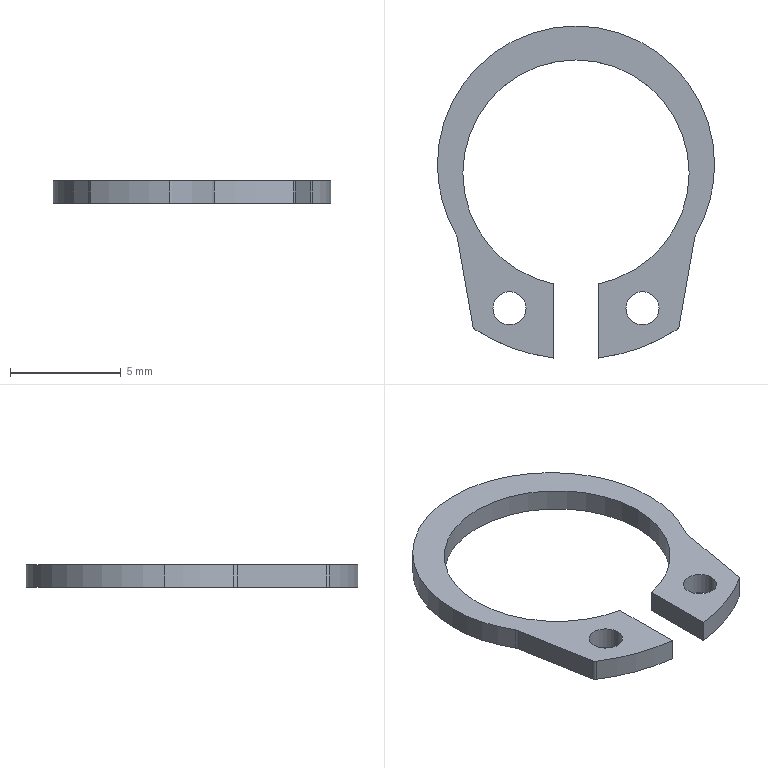Part | SolidWorks | features MoveCopyBody 1, Stock 1 | 1 solid | 22 faces | box 12.5 x 14.97 x 1 mm | volume 58.29 mm3 | cylinder 16 | plane 6 | commonest cylinder face diameters 1.5 x4 10.2 x3 12.5 x3 0.4 x2 1 x2 16.8 x2
STEP:
#1=CARTESIAN_POINT('',(2.25,-6.102,0.));
#2=VERTEX_POINT('',#1);
#3=CARTESIAN_POINT('',(3.75,-6.102,0.));
#4=VERTEX_POINT('',#3);
#5=CARTESIAN_POINT('',(3.,-6.102,0.));
#6=DIRECTION('',(0.,0.,1.));
#7=DIRECTION('',(-1.,0.,0.));
#8=AXIS2_PLACEMENT_3D('',#5,#6,#7);
#9=CIRCLE('',#8,0.75);
#10=EDGE_CURVE('',#2,#4,#9,.T.);
#11=ORIENTED_EDGE('',*,*,#10,.F.);
#12=CARTESIAN_POINT('',(2.25,-6.102,1.));
#13=VERTEX_POINT('',#12);
#14=CARTESIAN_POINT('',(2.25,-6.102,0.));
#15=DIRECTION('',(0.,0.,1.));
#16=VECTOR('',#15,1000.);
#17=LINE('',#14,#16);
#18=EDGE_CURVE('',#2,#13,#17,.T.);
#19=ORIENTED_EDGE('',*,*,#18,.T.);
#20=CARTESIAN_POINT('',(3.75,-6.102,1.));
#21=VERTEX_POINT('',#20);
#22=CARTESIAN_POINT('',(3.,-6.102,1.));
#23=DIRECTION('',(0.,0.,1.));
#24=DIRECTION('',(-1.,0.,0.));
#25=AXIS2_PLACEMENT_3D('',#22,#23,#24);
#26=CIRCLE('',#25,0.75);
#27=EDGE_CURVE('',#13,#21,#26,.T.);
#28=ORIENTED_EDGE('',*,*,#27,.T.);
#29=CARTESIAN_POINT('',(3.75,-6.102,0.));
#30=DIRECTION('',(0.,0.,1.));
#31=VECTOR('',#30,1000.);
#32=LINE('',#29,#31);
#33=EDGE_CURVE('',#4,#21,#32,.T.);
#34=ORIENTED_EDGE('',*,*,#33,.F.);
#35=EDGE_LOOP('',(#11,#19,#28,#34));
#36=FACE_OUTER_BOUND('',#35,.T.);
#37=CARTESIAN_POINT('',(3.,-6.102,0.));
#38=DIRECTION('',(0.,0.,1.));
#39=DIRECTION('',(1.,0.,0.));
#40=AXIS2_PLACEMENT_3D('',#37,#38,#39);
#41=CYLINDRICAL_SURFACE('',#40,0.75);
#42=ADVANCED_FACE('',(#36),#41,.F.);
#43=CARTESIAN_POINT('',(-3.75,-6.102,0.));
#44=VERTEX_POINT('',#43);
#45=CARTESIAN_POINT('',(-2.25,-6.102,0.));
#46=VERTEX_POINT('',#45);
#47=CARTESIAN_POINT('',(-3.,-6.102,0.));
#48=DIRECTION('',(0.,0.,1.));
#49=DIRECTION('',(1.,0.,0.));
#50=AXIS2_PLACEMENT_3D('',#47,#48,#49);
#51=CIRCLE('',#50,0.75);
#52=EDGE_CURVE('',#44,#46,#51,.T.);
#53=ORIENTED_EDGE('',*,*,#52,.F.);
#54=CARTESIAN_POINT('',(-3.75,-6.102,1.));
#55=VERTEX_POINT('',#54);
#56=CARTESIAN_POINT('',(-3.75,-6.102,0.));
#57=DIRECTION('',(0.,0.,1.));
#58=VECTOR('',#57,1000.);
#59=LINE('',#56,#58);
#60=EDGE_CURVE('',#44,#55,#59,.T.);
#61=ORIENTED_EDGE('',*,*,#60,.T.);
#62=CARTESIAN_POINT('',(-2.25,-6.102,1.));
#63=VERTEX_POINT('',#62);
#64=CARTESIAN_POINT('',(-3.,-6.102,1.));
#65=DIRECTION('',(0.,0.,1.));
#66=DIRECTION('',(1.,0.,0.));
#67=AXIS2_PLACEMENT_3D('',#64,#65,#66);
#68=CIRCLE('',#67,0.75);
#69=EDGE_CURVE('',#55,#63,#68,.T.);
#70=ORIENTED_EDGE('',*,*,#69,.T.);
#71=CARTESIAN_POINT('',(-2.25,-6.102,0.));
#72=DIRECTION('',(0.,0.,1.));
#73=VECTOR('',#72,1000.);
#74=LINE('',#71,#73);
#75=EDGE_CURVE('',#46,#63,#74,.T.);
#76=ORIENTED_EDGE('',*,*,#75,.F.);
#77=EDGE_LOOP('',(#53,#61,#70,#76));
#78=FACE_OUTER_BOUND('',#77,.T.);
#79=CARTESIAN_POINT('',(-3.,-6.102,0.));
#80=DIRECTION('',(0.,0.,1.));
#81=DIRECTION('',(1.,0.,0.));
#82=AXIS2_PLACEMENT_3D('',#79,#80,#81);
#83=CYLINDRICAL_SURFACE('',#82,0.75);
#84=ADVANCED_FACE('',(#78),#83,.F.);
#85=CARTESIAN_POINT('',(6.25,0.38,0.));
#86=VERTEX_POINT('',#85);
#87=CARTESIAN_POINT('',(-6.25,0.38,0.));
#88=VERTEX_POINT('',#87);
#89=CARTESIAN_POINT('',(0.,0.38,0.));
#90=DIRECTION('',(0.,0.,1.));
#91=DIRECTION('',(1.,0.,0.));
#92=AXIS2_PLACEMENT_3D('',#89,#90,#91);
#93=CIRCLE('',#92,6.25);
#94=EDGE_CURVE('',#86,#88,#93,.T.);
#95=ORIENTED_EDGE('',*,*,#94,.T.);
#96=CARTESIAN_POINT('',(-6.25,0.38,1.));
#97=VERTEX_POINT('',#96);
#98=CARTESIAN_POINT('',(-6.25,0.38,0.));
#99=DIRECTION('',(0.,0.,1.));
#100=VECTOR('',#99,1000.);
#101=LINE('',#98,#100);
#102=EDGE_CURVE('',#88,#97,#101,.T.);
#103=ORIENTED_EDGE('',*,*,#102,.T.);
#104=CARTESIAN_POINT('',(6.25,0.38,1.));
#105=VERTEX_POINT('',#104);
#106=CARTESIAN_POINT('',(0.,0.38,1.));
#107=DIRECTION('',(0.,0.,1.));
#108=DIRECTION('',(1.,0.,0.));
#109=AXIS2_PLACEMENT_3D('',#106,#107,#108);
#110=CIRCLE('',#109,6.25);
#111=EDGE_CURVE('',#105,#97,#110,.T.);
#112=ORIENTED_EDGE('',*,*,#111,.F.);
#113=CARTESIAN_POINT('',(6.25,0.38,0.));
#114=DIRECTION('',(0.,0.,1.));
#115=VECTOR('',#114,1000.);
#116=LINE('',#113,#115);
#117=EDGE_CURVE('',#86,#105,#116,.T.);
#118=ORIENTED_EDGE('',*,*,#117,.F.);
#119=EDGE_LOOP('',(#95,#103,#112,#118));
#120=FACE_OUTER_BOUND('',#119,.T.);
#121=CARTESIAN_POINT('',(0.,0.38,0.));
#122=DIRECTION('',(0.,0.,1.));
#123=DIRECTION('',(1.,0.,0.));
#124=AXIS2_PLACEMENT_3D('',#121,#122,#123);
#125=CYLINDRICAL_SURFACE('',#124,6.25);
#126=ADVANCED_FACE('',(#120),#125,.T.);
#127=CARTESIAN_POINT('',(5.413,-2.744,0.));
#128=VERTEX_POINT('',#127);
#129=CARTESIAN_POINT('',(0.,0.38,0.));
#130=DIRECTION('',(0.,0.,1.));
#131=DIRECTION('',(1.,0.,0.));
#132=AXIS2_PLACEMENT_3D('',#129,#130,#131);
#133=CIRCLE('',#132,6.25);
#134=EDGE_CURVE('',#128,#86,#133,.T.);
#135=ORIENTED_EDGE('',*,*,#134,.T.);
#136=ORIENTED_EDGE('',*,*,#117,.T.);
#137=CARTESIAN_POINT('',(5.413,-2.744,1.));
#138=VERTEX_POINT('',#137);
#139=CARTESIAN_POINT('',(0.,0.38,1.));
#140=DIRECTION('',(0.,0.,1.));
#141=DIRECTION('',(1.,0.,0.));
#142=AXIS2_PLACEMENT_3D('',#139,#140,#141);
#143=CIRCLE('',#142,6.25);
#144=EDGE_CURVE('',#138,#105,#143,.T.);
#145=ORIENTED_EDGE('',*,*,#144,.F.);
#146=CARTESIAN_POINT('',(5.413,-2.744,0.));
#147=DIRECTION('',(0.,0.,-1.));
#148=VECTOR('',#147,1000.);
#149=LINE('',#146,#148);
#150=EDGE_CURVE('',#138,#128,#149,.T.);
#151=ORIENTED_EDGE('',*,*,#150,.T.);
#152=EDGE_LOOP('',(#135,#136,#145,#151));
#153=FACE_OUTER_BOUND('',#152,.T.);
#154=CARTESIAN_POINT('',(0.,0.38,0.));
#155=DIRECTION('',(0.,0.,1.));
#156=DIRECTION('',(1.,0.,0.));
#157=AXIS2_PLACEMENT_3D('',#154,#155,#156);
#158=CYLINDRICAL_SURFACE('',#157,6.25);
#159=ADVANCED_FACE('',(#153),#158,.T.);
#160=CARTESIAN_POINT('',(-1.,-5.001,0.));
#161=VERTEX_POINT('',#160);
#162=CARTESIAN_POINT('',(-5.1,0.,0.));
#163=VERTEX_POINT('',#162);
#164=CARTESIAN_POINT('',(0.,0.,0.));
#165=DIRECTION('',(0.,0.,-1.));
#166=DIRECTION('',(1.,0.,0.));
#167=AXIS2_PLACEMENT_3D('',#164,#165,#166);
#168=CIRCLE('',#167,5.1);
#169=EDGE_CURVE('',#161,#163,#168,.T.);
#170=ORIENTED_EDGE('',*,*,#169,.T.);
#171=CARTESIAN_POINT('',(-5.1,0.,1.));
#172=VERTEX_POINT('',#171);
#173=CARTESIAN_POINT('',(-5.1,0.,0.));
#174=DIRECTION('',(0.,0.,1.));
#175=VECTOR('',#174,1000.);
#176=LINE('',#173,#175);
#177=EDGE_CURVE('',#163,#172,#176,.T.);
#178=ORIENTED_EDGE('',*,*,#177,.T.);
#179=CARTESIAN_POINT('',(-1.,-5.001,1.));
#180=VERTEX_POINT('',#179);
#181=CARTESIAN_POINT('',(0.,0.,1.));
#182=DIRECTION('',(0.,0.,-1.));
#183=DIRECTION('',(1.,0.,0.));
#184=AXIS2_PLACEMENT_3D('',#181,#182,#183);
#185=CIRCLE('',#184,5.1);
#186=EDGE_CURVE('',#180,#172,#185,.T.);
#187=ORIENTED_EDGE('',*,*,#186,.F.);
#188=CARTESIAN_POINT('',(-1.,-5.001,0.));
#189=DIRECTION('',(0.,0.,1.));
#190=VECTOR('',#189,1000.);
#191=LINE('',#188,#190);
#192=EDGE_CURVE('',#161,#180,#191,.T.);
#193=ORIENTED_EDGE('',*,*,#192,.F.);
#194=EDGE_LOOP('',(#170,#178,#187,#193));
#195=FACE_OUTER_BOUND('',#194,.T.);
#196=CARTESIAN_POINT('',(0.,0.,0.));
#197=DIRECTION('',(0.,0.,1.));
#198=DIRECTION('',(1.,0.,0.));
#199=AXIS2_PLACEMENT_3D('',#196,#197,#198);
#200=CYLINDRICAL_SURFACE('',#199,5.1);
#201=ADVANCED_FACE('',(#195),#200,.F.);
#202=ORIENTED_EDGE('',*,*,#177,.F.);
#203=CARTESIAN_POINT('',(5.1,0.,0.));
#204=VERTEX_POINT('',#203);
#205=CARTESIAN_POINT('',(0.,0.,0.));
#206=DIRECTION('',(0.,0.,-1.));
#207=DIRECTION('',(1.,0.,0.));
#208=AXIS2_PLACEMENT_3D('',#205,#206,#207);
#209=CIRCLE('',#208,5.1);
#210=EDGE_CURVE('',#163,#204,#209,.T.);
#211=ORIENTED_EDGE('',*,*,#210,.T.);
#212=CARTESIAN_POINT('',(5.1,0.,1.));
#213=VERTEX_POINT('',#212);
#214=CARTESIAN_POINT('',(5.1,0.,0.));
#215=DIRECTION('',(0.,0.,1.));
#216=VECTOR('',#215,1000.);
#217=LINE('',#214,#216);
#218=EDGE_CURVE('',#204,#213,#217,.T.);
#219=ORIENTED_EDGE('',*,*,#218,.T.);
#220=CARTESIAN_POINT('',(0.,0.,1.));
#221=DIRECTION('',(0.,0.,-1.));
#222=DIRECTION('',(1.,0.,0.));
#223=AXIS2_PLACEMENT_3D('',#220,#221,#222);
#224=CIRCLE('',#223,5.1);
#225=EDGE_CURVE('',#172,#213,#224,.T.);
#226=ORIENTED_EDGE('',*,*,#225,.F.);
#227=EDGE_LOOP('',(#202,#211,#219,#226));
#228=FACE_OUTER_BOUND('',#227,.T.);
#229=CARTESIAN_POINT('',(0.,0.,0.));
#230=DIRECTION('',(0.,0.,1.));
#231=DIRECTION('',(1.,0.,0.));
#232=AXIS2_PLACEMENT_3D('',#229,#230,#231);
#233=CYLINDRICAL_SURFACE('',#232,5.1);
#234=ADVANCED_FACE('',(#228),#233,.F.);
#235=CARTESIAN_POINT('',(1.,-8.34,0.));
#236=VERTEX_POINT('',#235);
#237=CARTESIAN_POINT('',(4.557,-7.056,0.));
#238=VERTEX_POINT('',#237);
#239=CARTESIAN_POINT('',(0.,0.,0.));
#240=DIRECTION('',(0.,0.,1.));
#241=DIRECTION('',(-1.,0.,0.));
#242=AXIS2_PLACEMENT_3D('',#239,#240,#241);
#243=CIRCLE('',#242,8.4);
#244=EDGE_CURVE('',#236,#238,#243,.T.);
#245=ORIENTED_EDGE('',*,*,#244,.T.);
#246=CARTESIAN_POINT('',(4.557,-7.056,1.));
#247=VERTEX_POINT('',#246);
#248=CARTESIAN_POINT('',(4.557,-7.056,0.));
#249=DIRECTION('',(0.,0.,1.));
#250=VECTOR('',#249,1000.);
#251=LINE('',#248,#250);
#252=EDGE_CURVE('',#238,#247,#251,.T.);
#253=ORIENTED_EDGE('',*,*,#252,.T.);
#254=CARTESIAN_POINT('',(1.,-8.34,1.));
#255=VERTEX_POINT('',#254);
#256=CARTESIAN_POINT('',(0.,0.,1.));
#257=DIRECTION('',(0.,0.,1.));
#258=DIRECTION('',(-1.,0.,0.));
#259=AXIS2_PLACEMENT_3D('',#256,#257,#258);
#260=CIRCLE('',#259,8.4);
#261=EDGE_CURVE('',#255,#247,#260,.T.);
#262=ORIENTED_EDGE('',*,*,#261,.F.);
#263=CARTESIAN_POINT('',(1.,-8.34,0.));
#264=DIRECTION('',(0.,0.,1.));
#265=VECTOR('',#264,1000.);
#266=LINE('',#263,#265);
#267=EDGE_CURVE('',#236,#255,#266,.T.);
#268=ORIENTED_EDGE('',*,*,#267,.F.);
#269=EDGE_LOOP('',(#245,#253,#262,#268));
#270=FACE_OUTER_BOUND('',#269,.T.);
#271=CARTESIAN_POINT('',(0.,0.,0.));
#272=DIRECTION('',(0.,0.,1.));
#273=DIRECTION('',(1.,0.,0.));
#274=AXIS2_PLACEMENT_3D('',#271,#272,#273);
#275=CYLINDRICAL_SURFACE('',#274,8.4);
#276=ADVANCED_FACE('',(#270),#275,.T.);
#277=CARTESIAN_POINT('',(1.,-5.001,1.));
#278=VERTEX_POINT('',#277);
#279=CARTESIAN_POINT('',(1.,-5.001,1.));
#280=DIRECTION('',(0.,-1.,0.));
#281=VECTOR('',#280,1000.);
#282=LINE('',#279,#281);
#283=EDGE_CURVE('',#278,#255,#282,.T.);
#284=ORIENTED_EDGE('',*,*,#283,.F.);
#285=CARTESIAN_POINT('',(1.,-5.001,0.));
#286=VERTEX_POINT('',#285);
#287=CARTESIAN_POINT('',(1.,-5.001,0.));
#288=DIRECTION('',(0.,0.,1.));
#289=VECTOR('',#288,1000.);
#290=LINE('',#287,#289);
#291=EDGE_CURVE('',#286,#278,#290,.T.);
#292=ORIENTED_EDGE('',*,*,#291,.F.);
#293=CARTESIAN_POINT('',(1.,-5.001,0.));
#294=DIRECTION('',(0.,-1.,0.));
#295=VECTOR('',#294,1000.);
#296=LINE('',#293,#295);
#297=EDGE_CURVE('',#286,#236,#296,.T.);
#298=ORIENTED_EDGE('',*,*,#297,.T.);
#299=ORIENTED_EDGE('',*,*,#267,.T.);
#300=EDGE_LOOP('',(#284,#292,#298,#299));
#301=FACE_OUTER_BOUND('',#300,.T.);
#302=CARTESIAN_POINT('',(1.,-5.001,0.));
#303=DIRECTION('',(-1.,0.,0.));
#304=DIRECTION('',(0.,-1.,0.));
#305=AXIS2_PLACEMENT_3D('',#302,#303,#304);
#306=PLANE('',#305);
#307=ADVANCED_FACE('',(#301),#306,.T.);
#308=ORIENTED_EDGE('',*,*,#218,.F.);
#309=CARTESIAN_POINT('',(0.,0.,0.));
#310=DIRECTION('',(0.,0.,-1.));
#311=DIRECTION('',(1.,0.,0.));
#312=AXIS2_PLACEMENT_3D('',#309,#310,#311);
#313=CIRCLE('',#312,5.1);
#314=EDGE_CURVE('',#204,#286,#313,.T.);
#315=ORIENTED_EDGE('',*,*,#314,.T.);
#316=ORIENTED_EDGE('',*,*,#291,.T.);
#317=CARTESIAN_POINT('',(0.,0.,1.));
#318=DIRECTION('',(0.,0.,-1.));
#319=DIRECTION('',(1.,0.,0.));
#320=AXIS2_PLACEMENT_3D('',#317,#318,#319);
#321=CIRCLE('',#320,5.1);
#322=EDGE_CURVE('',#213,#278,#321,.T.);
#323=ORIENTED_EDGE('',*,*,#322,.F.);
#324=EDGE_LOOP('',(#308,#315,#316,#323));
#325=FACE_OUTER_BOUND('',#324,.T.);
#326=CARTESIAN_POINT('',(0.,0.,0.));
#327=DIRECTION('',(0.,0.,1.));
#328=DIRECTION('',(1.,0.,0.));
#329=AXIS2_PLACEMENT_3D('',#326,#327,#328);
#330=CYLINDRICAL_SURFACE('',#329,5.1);
#331=ADVANCED_FACE('',(#325),#330,.F.);
#332=CARTESIAN_POINT('',(-1.,-8.34,1.));
#333=VERTEX_POINT('',#332);
#334=CARTESIAN_POINT('',(-1.,-5.001,1.));
#335=DIRECTION('',(0.,1.,0.));
#336=VECTOR('',#335,1000.);
#337=LINE('',#334,#336);
#338=EDGE_CURVE('',#333,#180,#337,.T.);
#339=ORIENTED_EDGE('',*,*,#338,.F.);
#340=CARTESIAN_POINT('',(-1.,-8.34,0.));
#341=VERTEX_POINT('',#340);
#342=CARTESIAN_POINT('',(-1.,-8.34,0.));
#343=DIRECTION('',(0.,0.,1.));
#344=VECTOR('',#343,1000.);
#345=LINE('',#342,#344);
#346=EDGE_CURVE('',#341,#333,#345,.T.);
#347=ORIENTED_EDGE('',*,*,#346,.F.);
#348=CARTESIAN_POINT('',(-1.,-5.001,0.));
#349=DIRECTION('',(0.,1.,0.));
#350=VECTOR('',#349,1000.);
#351=LINE('',#348,#350);
#352=EDGE_CURVE('',#341,#161,#351,.T.);
#353=ORIENTED_EDGE('',*,*,#352,.T.);
#354=ORIENTED_EDGE('',*,*,#192,.T.);
#355=EDGE_LOOP('',(#339,#347,#353,#354));
#356=FACE_OUTER_BOUND('',#355,.T.);
#357=CARTESIAN_POINT('',(-1.,-5.001,0.));
#358=DIRECTION('',(1.,0.,0.));
#359=DIRECTION('',(0.,1.,0.));
#360=AXIS2_PLACEMENT_3D('',#357,#358,#359);
#361=PLANE('',#360);
#362=ADVANCED_FACE('',(#356),#361,.T.);
#363=CARTESIAN_POINT('',(-4.557,-7.056,1.));
#364=VERTEX_POINT('',#363);
#365=CARTESIAN_POINT('',(0.,0.,1.));
#366=DIRECTION('',(0.,0.,1.));
#367=DIRECTION('',(1.,0.,0.));
#368=AXIS2_PLACEMENT_3D('',#365,#366,#367);
#369=CIRCLE('',#368,8.4);
#370=EDGE_CURVE('',#364,#333,#369,.T.);
#371=ORIENTED_EDGE('',*,*,#370,.F.);
#372=CARTESIAN_POINT('',(-4.557,-7.056,0.));
#373=VERTEX_POINT('',#372);
#374=CARTESIAN_POINT('',(-4.557,-7.056,0.));
#375=DIRECTION('',(0.,0.,-1.));
#376=VECTOR('',#375,1000.);
#377=LINE('',#374,#376);
#378=EDGE_CURVE('',#364,#373,#377,.T.);
#379=ORIENTED_EDGE('',*,*,#378,.T.);
#380=CARTESIAN_POINT('',(0.,0.,0.));
#381=DIRECTION('',(0.,0.,1.));
#382=DIRECTION('',(1.,0.,0.));
#383=AXIS2_PLACEMENT_3D('',#380,#381,#382);
#384=CIRCLE('',#383,8.4);
#385=EDGE_CURVE('',#373,#341,#384,.T.);
#386=ORIENTED_EDGE('',*,*,#385,.T.);
#387=ORIENTED_EDGE('',*,*,#346,.T.);
#388=EDGE_LOOP('',(#371,#379,#386,#387));
#389=FACE_OUTER_BOUND('',#388,.T.);
#390=CARTESIAN_POINT('',(0.,0.,0.));
#391=DIRECTION('',(0.,0.,1.));
#392=DIRECTION('',(1.,0.,0.));
#393=AXIS2_PLACEMENT_3D('',#390,#391,#392);
#394=CYLINDRICAL_SURFACE('',#393,8.4);
#395=ADVANCED_FACE('',(#389),#394,.T.);
#396=CARTESIAN_POINT('',(-5.354,-2.907,1.));
#397=VERTEX_POINT('',#396);
#398=CARTESIAN_POINT('',(-4.646,-6.923,1.));
#399=VERTEX_POINT('',#398);
#400=CARTESIAN_POINT('',(-5.369,-2.819,1.));
#401=DIRECTION('',(0.1736,-0.9848,0.));
#402=VECTOR('',#401,1000.);
#403=LINE('',#400,#402);
#404=EDGE_CURVE('',#397,#399,#403,.T.);
#405=ORIENTED_EDGE('',*,*,#404,.F.);
#406=CARTESIAN_POINT('',(-5.354,-2.907,0.));
#407=VERTEX_POINT('',#406);
#408=CARTESIAN_POINT('',(-5.354,-2.907,0.));
#409=DIRECTION('',(0.,0.,-1.));
#410=VECTOR('',#409,1000.);
#411=LINE('',#408,#410);
#412=EDGE_CURVE('',#397,#407,#411,.T.);
#413=ORIENTED_EDGE('',*,*,#412,.T.);
#414=CARTESIAN_POINT('',(-4.646,-6.923,0.));
#415=VERTEX_POINT('',#414);
#416=CARTESIAN_POINT('',(-5.369,-2.819,0.));
#417=DIRECTION('',(0.1736,-0.9848,0.));
#418=VECTOR('',#417,1000.);
#419=LINE('',#416,#418);
#420=EDGE_CURVE('',#407,#415,#419,.T.);
#421=ORIENTED_EDGE('',*,*,#420,.T.);
#422=CARTESIAN_POINT('',(-4.646,-6.923,0.));
#423=DIRECTION('',(0.,0.,1.));
#424=VECTOR('',#423,1000.);
#425=LINE('',#422,#424);
#426=EDGE_CURVE('',#415,#399,#425,.T.);
#427=ORIENTED_EDGE('',*,*,#426,.T.);
#428=EDGE_LOOP('',(#405,#413,#421,#427));
#429=FACE_OUTER_BOUND('',#428,.T.);
#430=CARTESIAN_POINT('',(-5.369,-2.819,0.));
#431=DIRECTION('',(-0.9848,-0.1736,0.));
#432=DIRECTION('',(0.1736,-0.9848,0.));
#433=AXIS2_PLACEMENT_3D('',#430,#431,#432);
#434=PLANE('',#433);
#435=ADVANCED_FACE('',(#429),#434,.T.);
#436=ORIENTED_EDGE('',*,*,#102,.F.);
#437=CARTESIAN_POINT('',(-5.413,-2.744,0.));
#438=VERTEX_POINT('',#437);
#439=CARTESIAN_POINT('',(0.,0.38,0.));
#440=DIRECTION('',(0.,0.,1.));
#441=DIRECTION('',(1.,0.,0.));
#442=AXIS2_PLACEMENT_3D('',#439,#440,#441);
#443=CIRCLE('',#442,6.25);
#444=EDGE_CURVE('',#88,#438,#443,.T.);
#445=ORIENTED_EDGE('',*,*,#444,.T.);
#446=CARTESIAN_POINT('',(-5.413,-2.744,1.));
#447=VERTEX_POINT('',#446);
#448=CARTESIAN_POINT('',(-5.413,-2.744,0.));
#449=DIRECTION('',(0.,0.,1.));
#450=VECTOR('',#449,1000.);
#451=LINE('',#448,#450);
#452=EDGE_CURVE('',#438,#447,#451,.T.);
#453=ORIENTED_EDGE('',*,*,#452,.T.);
#454=CARTESIAN_POINT('',(0.,0.38,1.));
#455=DIRECTION('',(0.,0.,1.));
#456=DIRECTION('',(1.,0.,0.));
#457=AXIS2_PLACEMENT_3D('',#454,#455,#456);
#458=CIRCLE('',#457,6.25);
#459=EDGE_CURVE('',#97,#447,#458,.T.);
#460=ORIENTED_EDGE('',*,*,#459,.F.);
#461=EDGE_LOOP('',(#436,#445,#453,#460));
#462=FACE_OUTER_BOUND('',#461,.T.);
#463=CARTESIAN_POINT('',(0.,0.38,0.));
#464=DIRECTION('',(0.,0.,1.));
#465=DIRECTION('',(1.,0.,0.));
#466=AXIS2_PLACEMENT_3D('',#463,#464,#465);
#467=CYLINDRICAL_SURFACE('',#466,6.25);
#468=ADVANCED_FACE('',(#462),#467,.T.);
#469=CARTESIAN_POINT('',(4.646,-6.923,0.));
#470=VERTEX_POINT('',#469);
#471=CARTESIAN_POINT('',(5.354,-2.907,0.));
#472=VERTEX_POINT('',#471);
#473=CARTESIAN_POINT('',(5.369,-2.819,0.));
#474=DIRECTION('',(0.1736,0.9848,0.));
#475=VECTOR('',#474,1000.);
#476=LINE('',#473,#475);
#477=EDGE_CURVE('',#470,#472,#476,.T.);
#478=ORIENTED_EDGE('',*,*,#477,.T.);
#479=CARTESIAN_POINT('',(5.354,-2.907,1.));
#480=VERTEX_POINT('',#479);
#481=CARTESIAN_POINT('',(5.354,-2.907,1.));
#482=DIRECTION('',(0.,0.,1.));
#483=VECTOR('',#482,1000.);
#484=LINE('',#481,#483);
#485=EDGE_CURVE('',#472,#480,#484,.T.);
#486=ORIENTED_EDGE('',*,*,#485,.T.);
#487=CARTESIAN_POINT('',(4.646,-6.923,1.));
#488=VERTEX_POINT('',#487);
#489=CARTESIAN_POINT('',(5.369,-2.819,1.));
#490=DIRECTION('',(0.1736,0.9848,0.));
#491=VECTOR('',#490,1000.);
#492=LINE('',#489,#491);
#493=EDGE_CURVE('',#488,#480,#492,.T.);
#494=ORIENTED_EDGE('',*,*,#493,.F.);
#495=CARTESIAN_POINT('',(4.646,-6.923,0.));
#496=DIRECTION('',(0.,0.,-1.));
#497=VECTOR('',#496,1000.);
#498=LINE('',#495,#497);
#499=EDGE_CURVE('',#488,#470,#498,.T.);
#500=ORIENTED_EDGE('',*,*,#499,.T.);
#501=EDGE_LOOP('',(#478,#486,#494,#500));
#502=FACE_OUTER_BOUND('',#501,.T.);
#503=CARTESIAN_POINT('',(5.369,-2.819,0.));
#504=DIRECTION('',(0.9848,-0.1736,0.));
#505=DIRECTION('',(0.1736,0.9848,0.));
#506=AXIS2_PLACEMENT_3D('',#503,#504,#505);
#507=PLANE('',#506);
#508=ADVANCED_FACE('',(#502),#507,.T.);
#509=CARTESIAN_POINT('',(3.,-6.102,0.));
#510=DIRECTION('',(0.,0.,1.));
#511=DIRECTION('',(-1.,0.,0.));
#512=AXIS2_PLACEMENT_3D('',#509,#510,#511);
#513=CIRCLE('',#512,0.75);
#514=EDGE_CURVE('',#4,#2,#513,.T.);
#515=ORIENTED_EDGE('',*,*,#514,.T.);
#516=ORIENTED_EDGE('',*,*,#10,.T.);
#517=EDGE_LOOP('',(#515,#516));
#518=FACE_BOUND('',#517,.T.);
#519=CARTESIAN_POINT('',(-3.,-6.102,0.));
#520=DIRECTION('',(0.,0.,1.));
#521=DIRECTION('',(1.,0.,0.));
#522=AXIS2_PLACEMENT_3D('',#519,#520,#521);
#523=CIRCLE('',#522,0.75);
#524=EDGE_CURVE('',#46,#44,#523,.T.);
#525=ORIENTED_EDGE('',*,*,#524,.T.);
#526=ORIENTED_EDGE('',*,*,#52,.T.);
#527=EDGE_LOOP('',(#525,#526));
#528=FACE_BOUND('',#527,.T.);
#529=ORIENTED_EDGE('',*,*,#385,.F.);
#530=CARTESIAN_POINT('',(-4.449,-6.888,0.));
#531=DIRECTION('',(0.,0.,-1.));
#532=DIRECTION('',(-1.,0.,0.));
#533=AXIS2_PLACEMENT_3D('',#530,#531,#532);
#534=CIRCLE('',#533,0.2);
#535=EDGE_CURVE('',#373,#415,#534,.T.);
#536=ORIENTED_EDGE('',*,*,#535,.T.);
#537=ORIENTED_EDGE('',*,*,#420,.F.);
#538=CARTESIAN_POINT('',(-5.846,-2.994,0.));
#539=DIRECTION('',(0.,0.,1.));
#540=DIRECTION('',(-1.,0.,0.));
#541=AXIS2_PLACEMENT_3D('',#538,#539,#540);
#542=CIRCLE('',#541,0.5);
#543=EDGE_CURVE('',#407,#438,#542,.T.);
#544=ORIENTED_EDGE('',*,*,#543,.T.);
#545=ORIENTED_EDGE('',*,*,#444,.F.);
#546=ORIENTED_EDGE('',*,*,#94,.F.);
#547=ORIENTED_EDGE('',*,*,#134,.F.);
#548=CARTESIAN_POINT('',(5.846,-2.994,0.));
#549=DIRECTION('',(0.,0.,1.));
#550=DIRECTION('',(-1.,0.,0.));
#551=AXIS2_PLACEMENT_3D('',#548,#549,#550);
#552=CIRCLE('',#551,0.5);
#553=EDGE_CURVE('',#128,#472,#552,.T.);
#554=ORIENTED_EDGE('',*,*,#553,.T.);
#555=ORIENTED_EDGE('',*,*,#477,.F.);
#556=CARTESIAN_POINT('',(4.449,-6.888,0.));
#557=DIRECTION('',(0.,0.,-1.));
#558=DIRECTION('',(-1.,0.,0.));
#559=AXIS2_PLACEMENT_3D('',#556,#557,#558);
#560=CIRCLE('',#559,0.2);
#561=EDGE_CURVE('',#470,#238,#560,.T.);
#562=ORIENTED_EDGE('',*,*,#561,.T.);
#563=ORIENTED_EDGE('',*,*,#244,.F.);
#564=ORIENTED_EDGE('',*,*,#297,.F.);
#565=ORIENTED_EDGE('',*,*,#314,.F.);
#566=ORIENTED_EDGE('',*,*,#210,.F.);
#567=ORIENTED_EDGE('',*,*,#169,.F.);
#568=ORIENTED_EDGE('',*,*,#352,.F.);
#569=EDGE_LOOP('',(#529,#536,#537,#544,#545,#546,#547,#554,#555,#562,#563,#564,#565,#566,#567,#568));
#570=FACE_OUTER_BOUND('',#569,.T.);
#571=CARTESIAN_POINT('',(0.,0.,0.));
#572=DIRECTION('',(0.,0.,-1.));
#573=DIRECTION('',(-1.,0.,0.));
#574=AXIS2_PLACEMENT_3D('',#571,#572,#573);
#575=PLANE('',#574);
#576=ADVANCED_FACE('',(#518,#528,#570),#575,.T.);
#577=CARTESIAN_POINT('',(3.,-6.102,1.));
#578=DIRECTION('',(0.,0.,1.));
#579=DIRECTION('',(-1.,0.,0.));
#580=AXIS2_PLACEMENT_3D('',#577,#578,#579);
#581=CIRCLE('',#580,0.75);
#582=EDGE_CURVE('',#21,#13,#581,.T.);
#583=ORIENTED_EDGE('',*,*,#582,.F.);
#584=ORIENTED_EDGE('',*,*,#27,.F.);
#585=EDGE_LOOP('',(#583,#584));
#586=FACE_BOUND('',#585,.T.);
#587=CARTESIAN_POINT('',(-3.,-6.102,1.));
#588=DIRECTION('',(0.,0.,1.));
#589=DIRECTION('',(1.,0.,0.));
#590=AXIS2_PLACEMENT_3D('',#587,#588,#589);
#591=CIRCLE('',#590,0.75);
#592=EDGE_CURVE('',#63,#55,#591,.T.);
#593=ORIENTED_EDGE('',*,*,#592,.F.);
#594=ORIENTED_EDGE('',*,*,#69,.F.);
#595=EDGE_LOOP('',(#593,#594));
#596=FACE_BOUND('',#595,.T.);
#597=ORIENTED_EDGE('',*,*,#144,.T.);
#598=ORIENTED_EDGE('',*,*,#111,.T.);
#599=ORIENTED_EDGE('',*,*,#459,.T.);
#600=CARTESIAN_POINT('',(-5.846,-2.994,1.));
#601=DIRECTION('',(0.,0.,-1.));
#602=DIRECTION('',(-1.,0.,0.));
#603=AXIS2_PLACEMENT_3D('',#600,#601,#602);
#604=CIRCLE('',#603,0.5);
#605=EDGE_CURVE('',#447,#397,#604,.T.);
#606=ORIENTED_EDGE('',*,*,#605,.T.);
#607=ORIENTED_EDGE('',*,*,#404,.T.);
#608=CARTESIAN_POINT('',(-4.449,-6.888,1.));
#609=DIRECTION('',(0.,0.,1.));
#610=DIRECTION('',(-1.,0.,0.));
#611=AXIS2_PLACEMENT_3D('',#608,#609,#610);
#612=CIRCLE('',#611,0.2);
#613=EDGE_CURVE('',#399,#364,#612,.T.);
#614=ORIENTED_EDGE('',*,*,#613,.T.);
#615=ORIENTED_EDGE('',*,*,#370,.T.);
#616=ORIENTED_EDGE('',*,*,#338,.T.);
#617=ORIENTED_EDGE('',*,*,#186,.T.);
#618=ORIENTED_EDGE('',*,*,#225,.T.);
#619=ORIENTED_EDGE('',*,*,#322,.T.);
#620=ORIENTED_EDGE('',*,*,#283,.T.);
#621=ORIENTED_EDGE('',*,*,#261,.T.);
#622=CARTESIAN_POINT('',(4.449,-6.888,1.));
#623=DIRECTION('',(0.,0.,1.));
#624=DIRECTION('',(-1.,0.,0.));
#625=AXIS2_PLACEMENT_3D('',#622,#623,#624);
#626=CIRCLE('',#625,0.2);
#627=EDGE_CURVE('',#247,#488,#626,.T.);
#628=ORIENTED_EDGE('',*,*,#627,.T.);
#629=ORIENTED_EDGE('',*,*,#493,.T.);
#630=CARTESIAN_POINT('',(5.846,-2.994,1.));
#631=DIRECTION('',(0.,0.,-1.));
#632=DIRECTION('',(-1.,0.,0.));
#633=AXIS2_PLACEMENT_3D('',#630,#631,#632);
#634=CIRCLE('',#633,0.5);
#635=EDGE_CURVE('',#480,#138,#634,.T.);
#636=ORIENTED_EDGE('',*,*,#635,.T.);
#637=EDGE_LOOP('',(#597,#598,#599,#606,#607,#614,#615,#616,#617,#618,#619,#620,#621,#628,#629,#636));
#638=FACE_OUTER_BOUND('',#637,.T.);
#639=CARTESIAN_POINT('',(0.,0.,1.));
#640=DIRECTION('',(0.,0.,-1.));
#641=DIRECTION('',(-1.,0.,0.));
#642=AXIS2_PLACEMENT_3D('',#639,#640,#641);
#643=PLANE('',#642);
#644=ADVANCED_FACE('',(#586,#596,#638),#643,.F.);
#645=ORIENTED_EDGE('',*,*,#60,.F.);
#646=ORIENTED_EDGE('',*,*,#524,.F.);
#647=ORIENTED_EDGE('',*,*,#75,.T.);
#648=ORIENTED_EDGE('',*,*,#592,.T.);
#649=EDGE_LOOP('',(#645,#646,#647,#648));
#650=FACE_OUTER_BOUND('',#649,.T.);
#651=CARTESIAN_POINT('',(-3.,-6.102,0.));
#652=DIRECTION('',(0.,0.,1.));
#653=DIRECTION('',(1.,0.,0.));
#654=AXIS2_PLACEMENT_3D('',#651,#652,#653);
#655=CYLINDRICAL_SURFACE('',#654,0.75);
#656=ADVANCED_FACE('',(#650),#655,.F.);
#657=ORIENTED_EDGE('',*,*,#18,.F.);
#658=ORIENTED_EDGE('',*,*,#514,.F.);
#659=ORIENTED_EDGE('',*,*,#33,.T.);
#660=ORIENTED_EDGE('',*,*,#582,.T.);
#661=EDGE_LOOP('',(#657,#658,#659,#660));
#662=FACE_OUTER_BOUND('',#661,.T.);
#663=CARTESIAN_POINT('',(3.,-6.102,0.));
#664=DIRECTION('',(0.,0.,1.));
#665=DIRECTION('',(1.,0.,0.));
#666=AXIS2_PLACEMENT_3D('',#663,#664,#665);
#667=CYLINDRICAL_SURFACE('',#666,0.75);
#668=ADVANCED_FACE('',(#662),#667,.F.);
#669=ORIENTED_EDGE('',*,*,#535,.F.);
#670=ORIENTED_EDGE('',*,*,#378,.F.);
#671=ORIENTED_EDGE('',*,*,#613,.F.);
#672=ORIENTED_EDGE('',*,*,#426,.F.);
#673=EDGE_LOOP('',(#669,#670,#671,#672));
#674=FACE_OUTER_BOUND('',#673,.T.);
#675=CARTESIAN_POINT('',(-4.449,-6.888,0.));
#676=DIRECTION('',(0.,0.,1.));
#677=DIRECTION('',(1.,0.,0.));
#678=AXIS2_PLACEMENT_3D('',#675,#676,#677);
#679=CYLINDRICAL_SURFACE('',#678,0.2);
#680=ADVANCED_FACE('',(#674),#679,.T.);
#681=ORIENTED_EDGE('',*,*,#561,.F.);
#682=ORIENTED_EDGE('',*,*,#499,.F.);
#683=ORIENTED_EDGE('',*,*,#627,.F.);
#684=ORIENTED_EDGE('',*,*,#252,.F.);
#685=EDGE_LOOP('',(#681,#682,#683,#684));
#686=FACE_OUTER_BOUND('',#685,.T.);
#687=CARTESIAN_POINT('',(4.449,-6.888,0.));
#688=DIRECTION('',(0.,0.,1.));
#689=DIRECTION('',(1.,0.,0.));
#690=AXIS2_PLACEMENT_3D('',#687,#688,#689);
#691=CYLINDRICAL_SURFACE('',#690,0.2);
#692=ADVANCED_FACE('',(#686),#691,.T.);
#693=ORIENTED_EDGE('',*,*,#553,.F.);
#694=ORIENTED_EDGE('',*,*,#150,.F.);
#695=ORIENTED_EDGE('',*,*,#635,.F.);
#696=ORIENTED_EDGE('',*,*,#485,.F.);
#697=EDGE_LOOP('',(#693,#694,#695,#696));
#698=FACE_OUTER_BOUND('',#697,.T.);
#699=CARTESIAN_POINT('',(5.846,-2.994,0.));
#700=DIRECTION('',(0.,0.,1.));
#701=DIRECTION('',(1.,0.,0.));
#702=AXIS2_PLACEMENT_3D('',#699,#700,#701);
#703=CYLINDRICAL_SURFACE('',#702,0.5);
#704=ADVANCED_FACE('',(#698),#703,.F.);
#705=ORIENTED_EDGE('',*,*,#543,.F.);
#706=ORIENTED_EDGE('',*,*,#412,.F.);
#707=ORIENTED_EDGE('',*,*,#605,.F.);
#708=ORIENTED_EDGE('',*,*,#452,.F.);
#709=EDGE_LOOP('',(#705,#706,#707,#708));
#710=FACE_OUTER_BOUND('',#709,.T.);
#711=CARTESIAN_POINT('',(-5.846,-2.994,0.));
#712=DIRECTION('',(0.,0.,1.));
#713=DIRECTION('',(1.,0.,0.));
#714=AXIS2_PLACEMENT_3D('',#711,#712,#713);
#715=CYLINDRICAL_SURFACE('',#714,0.5);
#716=ADVANCED_FACE('',(#710),#715,.F.);
#717=CLOSED_SHELL('',(#42,#84,#126,#159,#201,#234,#276,#307,#331,#362,#395,#435,#468,#508,#576,#644,#656,#668,#680,#692,#704,#716));
#718=MANIFOLD_SOLID_BREP('',#717);
#719=CARTESIAN_POINT('',(0.,0.,0.));
#720=DIRECTION('',(0.,0.,1.));
#721=DIRECTION('',(1.,0.,0.));
#722=AXIS2_PLACEMENT_3D('',#719,#720,#721);
#723=(LENGTH_UNIT()NAMED_UNIT(*)SI_UNIT(.MILLI.,.METRE.));
#724=UNCERTAINTY_MEASURE_WITH_UNIT(LENGTH_MEASURE(0.00001),#723,'','');
#725=(NAMED_UNIT(*)PLANE_ANGLE_UNIT()SI_UNIT($,.RADIAN.));
#726=(NAMED_UNIT(*)SI_UNIT($,.STERADIAN.)SOLID_ANGLE_UNIT());
#727=(GEOMETRIC_REPRESENTATION_CONTEXT(3)GLOBAL_UNCERTAINTY_ASSIGNED_CONTEXT((#724))GLOBAL_UNIT_ASSIGNED_CONTEXT((#723,#725,#726))REPRESENTATION_CONTEXT('',''));
#728=ADVANCED_BREP_SHAPE_REPRESENTATION('',(#718,#722),#727);